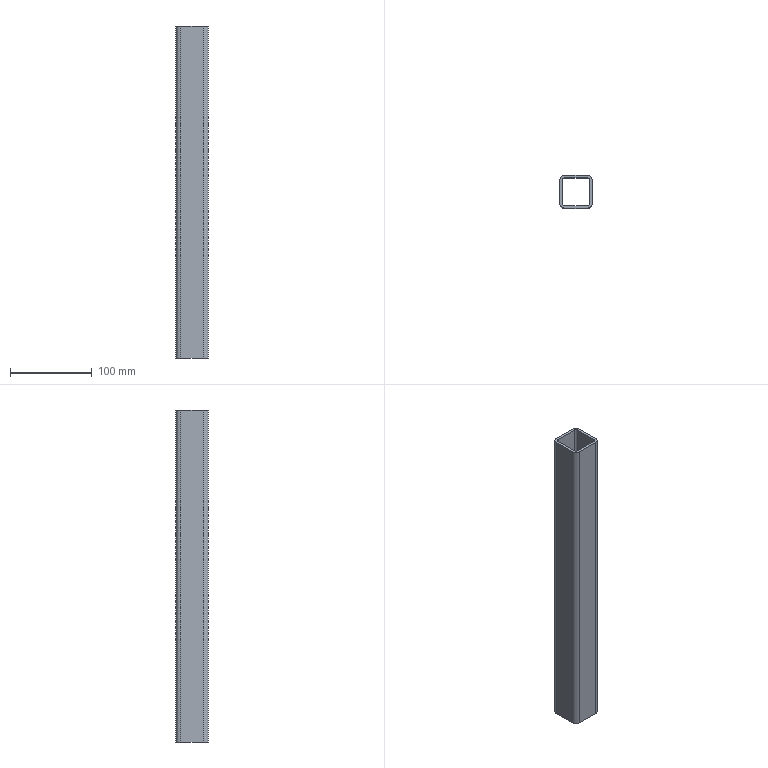Part | STEP file | SN10_003_008-08_TUBO_QUADRADO | 1 solid | 18 faces | box 40 x 40 x 407 mm | volume 171275 mm3 | plane 10 | cylinder 8 | commonest cylinder face diameters 6 x4 12 x4
STEP:
#1=CARTESIAN_POINT('',(0.,0.,0.));
#2=DIRECTION('',(0.,0.,1.));
#3=DIRECTION('',(1.,0.,0.));
#4=AXIS2_PLACEMENT_3D('',#1,#2,#3);
#5=CARTESIAN_POINT('',(2332.,-174.,20.));
#6=VERTEX_POINT('',#5);
#7=CARTESIAN_POINT('',(2326.,-180.,20.));
#8=VERTEX_POINT('',#7);
#9=CARTESIAN_POINT('',(2326.,-174.,20.));
#10=DIRECTION('',(0.,0.,-1.));
#11=DIRECTION('',(1.,0.,0.));
#12=AXIS2_PLACEMENT_3D('',#9,#10,#11);
#13=CIRCLE('',#12,6.);
#14=CARTESIAN_POINT('',(0.,0.,20.));
#15=DIRECTION('',(0.,0.,-1.));
#16=DIRECTION('',(-1.,0.,0.));
#17=AXIS2_PLACEMENT_3D('',#14,#15,#16);
#18=PLANE('',#17);
#19=CARTESIAN_POINT('',(-2326.,-174.));
#20=DIRECTION('',(-1.,0.));
#21=AXIS2_PLACEMENT_2D('',#19,#20);
#22=CIRCLE('',#21,6.);
#23=(GEOMETRIC_REPRESENTATION_CONTEXT(2)PARAMETRIC_REPRESENTATION_CONTEXT()REPRESENTATION_CONTEXT('',''));
#24=DEFINITIONAL_REPRESENTATION('',(#22),#23);
#25=PCURVE('',#18,#24);
#26=CARTESIAN_POINT('',(2326.,-174.,224.11));
#27=DIRECTION('',(0.,0.,-1.));
#28=DIRECTION('',(1.,0.,0.));
#29=AXIS2_PLACEMENT_3D('',#26,#27,#28);
#30=CYLINDRICAL_SURFACE('',#29,6.);
#31=CARTESIAN_POINT('',(0.,204.11));
#32=DIRECTION('',(1.,0.));
#33=VECTOR('',#32,1.);
#34=LINE('',#31,#33);
#35=(GEOMETRIC_REPRESENTATION_CONTEXT(2)PARAMETRIC_REPRESENTATION_CONTEXT()REPRESENTATION_CONTEXT('',''));
#36=DEFINITIONAL_REPRESENTATION('',(#34),#35);
#37=PCURVE('',#30,#36);
#38=SURFACE_CURVE('',#13,(#25,#37),.PCURVE_S1.);
#39=EDGE_CURVE('',#6,#8,#38,.T.);
#40=ORIENTED_EDGE('',*,*,#39,.T.);
#41=CARTESIAN_POINT('',(2298.,-180.,20.));
#42=VERTEX_POINT('',#41);
#43=CARTESIAN_POINT('',(2298.,-180.,20.));
#44=DIRECTION('',(1.,0.,0.));
#45=VECTOR('',#44,1.);
#46=LINE('',#43,#45);
#47=CARTESIAN_POINT('',(-2298.,-180.));
#48=DIRECTION('',(-1.,0.));
#49=VECTOR('',#48,1.);
#50=LINE('',#47,#49);
#51=(GEOMETRIC_REPRESENTATION_CONTEXT(2)PARAMETRIC_REPRESENTATION_CONTEXT()REPRESENTATION_CONTEXT('',''));
#52=DEFINITIONAL_REPRESENTATION('',(#50),#51);
#53=PCURVE('',#18,#52);
#54=CARTESIAN_POINT('',(2298.,-180.,20.));
#55=DIRECTION('',(0.,-1.,0.));
#56=DIRECTION('',(0.,0.,-1.));
#57=AXIS2_PLACEMENT_3D('',#54,#55,#56);
#58=PLANE('',#57);
#59=CARTESIAN_POINT('',(0.,0.));
#60=DIRECTION('',(0.,1.));
#61=VECTOR('',#60,1.);
#62=LINE('',#59,#61);
#63=(GEOMETRIC_REPRESENTATION_CONTEXT(2)PARAMETRIC_REPRESENTATION_CONTEXT()REPRESENTATION_CONTEXT('',''));
#64=DEFINITIONAL_REPRESENTATION('',(#62),#63);
#65=PCURVE('',#58,#64);
#66=SURFACE_CURVE('',#46,(#53,#65),.PCURVE_S1.);
#67=EDGE_CURVE('',#42,#8,#66,.T.);
#68=ORIENTED_EDGE('',*,*,#67,.F.);
#69=CARTESIAN_POINT('',(2292.,-174.,20.));
#70=VERTEX_POINT('',#69);
#71=CARTESIAN_POINT('',(2298.,-174.,20.));
#72=DIRECTION('',(0.,0.,-1.));
#73=DIRECTION('',(1.,0.,0.));
#74=AXIS2_PLACEMENT_3D('',#71,#72,#73);
#75=CIRCLE('',#74,6.);
#76=CARTESIAN_POINT('',(-2298.,-174.));
#77=DIRECTION('',(-1.,0.));
#78=AXIS2_PLACEMENT_2D('',#76,#77);
#79=CIRCLE('',#78,6.);
#80=(GEOMETRIC_REPRESENTATION_CONTEXT(2)PARAMETRIC_REPRESENTATION_CONTEXT()REPRESENTATION_CONTEXT('',''));
#81=DEFINITIONAL_REPRESENTATION('',(#79),#80);
#82=PCURVE('',#18,#81);
#83=CARTESIAN_POINT('',(2298.,-174.,224.11));
#84=DIRECTION('',(0.,0.,-1.));
#85=DIRECTION('',(0.,-1.,0.));
#86=AXIS2_PLACEMENT_3D('',#83,#84,#85);
#87=CYLINDRICAL_SURFACE('',#86,6.);
#88=CARTESIAN_POINT('',(-1.571,204.11));
#89=DIRECTION('',(1.,0.));
#90=VECTOR('',#89,1.);
#91=LINE('',#88,#90);
#92=(GEOMETRIC_REPRESENTATION_CONTEXT(2)PARAMETRIC_REPRESENTATION_CONTEXT()REPRESENTATION_CONTEXT('',''));
#93=DEFINITIONAL_REPRESENTATION('',(#91),#92);
#94=PCURVE('',#87,#93);
#95=SURFACE_CURVE('',#75,(#82,#94),.PCURVE_S1.);
#96=EDGE_CURVE('',#42,#70,#95,.T.);
#97=ORIENTED_EDGE('',*,*,#96,.T.);
#98=CARTESIAN_POINT('',(2292.,-146.,20.));
#99=VERTEX_POINT('',#98);
#100=CARTESIAN_POINT('',(2292.,-146.,20.));
#101=DIRECTION('',(0.,-1.,0.));
#102=VECTOR('',#101,1.);
#103=LINE('',#100,#102);
#104=CARTESIAN_POINT('',(-2292.,-146.));
#105=DIRECTION('',(0.,-1.));
#106=VECTOR('',#105,1.);
#107=LINE('',#104,#106);
#108=(GEOMETRIC_REPRESENTATION_CONTEXT(2)PARAMETRIC_REPRESENTATION_CONTEXT()REPRESENTATION_CONTEXT('',''));
#109=DEFINITIONAL_REPRESENTATION('',(#107),#108);
#110=PCURVE('',#18,#109);
#111=CARTESIAN_POINT('',(2292.,-146.,20.));
#112=DIRECTION('',(-1.,0.,0.));
#113=DIRECTION('',(0.,0.,1.));
#114=AXIS2_PLACEMENT_3D('',#111,#112,#113);
#115=PLANE('',#114);
#116=CARTESIAN_POINT('',(0.,0.));
#117=DIRECTION('',(0.,-1.));
#118=VECTOR('',#117,1.);
#119=LINE('',#116,#118);
#120=(GEOMETRIC_REPRESENTATION_CONTEXT(2)PARAMETRIC_REPRESENTATION_CONTEXT()REPRESENTATION_CONTEXT('',''));
#121=DEFINITIONAL_REPRESENTATION('',(#119),#120);
#122=PCURVE('',#115,#121);
#123=SURFACE_CURVE('',#103,(#110,#122),.PCURVE_S1.);
#124=EDGE_CURVE('',#99,#70,#123,.T.);
#125=ORIENTED_EDGE('',*,*,#124,.F.);
#126=CARTESIAN_POINT('',(2298.,-140.,20.));
#127=VERTEX_POINT('',#126);
#128=CARTESIAN_POINT('',(2298.,-146.,20.));
#129=DIRECTION('',(0.,0.,-1.));
#130=DIRECTION('',(1.,0.,0.));
#131=AXIS2_PLACEMENT_3D('',#128,#129,#130);
#132=CIRCLE('',#131,6.);
#133=CARTESIAN_POINT('',(-2298.,-146.));
#134=DIRECTION('',(-1.,0.));
#135=AXIS2_PLACEMENT_2D('',#133,#134);
#136=CIRCLE('',#135,6.);
#137=(GEOMETRIC_REPRESENTATION_CONTEXT(2)PARAMETRIC_REPRESENTATION_CONTEXT()REPRESENTATION_CONTEXT('',''));
#138=DEFINITIONAL_REPRESENTATION('',(#136),#137);
#139=PCURVE('',#18,#138);
#140=CARTESIAN_POINT('',(2298.,-146.,224.11));
#141=DIRECTION('',(0.,0.,-1.));
#142=DIRECTION('',(-1.,0.,0.));
#143=AXIS2_PLACEMENT_3D('',#140,#141,#142);
#144=CYLINDRICAL_SURFACE('',#143,6.);
#145=CARTESIAN_POINT('',(-3.142,204.11));
#146=DIRECTION('',(1.,0.));
#147=VECTOR('',#146,1.);
#148=LINE('',#145,#147);
#149=(GEOMETRIC_REPRESENTATION_CONTEXT(2)PARAMETRIC_REPRESENTATION_CONTEXT()REPRESENTATION_CONTEXT('',''));
#150=DEFINITIONAL_REPRESENTATION('',(#148),#149);
#151=PCURVE('',#144,#150);
#152=SURFACE_CURVE('',#132,(#139,#151),.PCURVE_S1.);
#153=EDGE_CURVE('',#99,#127,#152,.T.);
#154=ORIENTED_EDGE('',*,*,#153,.T.);
#155=CARTESIAN_POINT('',(2326.,-140.,20.));
#156=VERTEX_POINT('',#155);
#157=CARTESIAN_POINT('',(2326.,-140.,20.));
#158=DIRECTION('',(-1.,0.,0.));
#159=VECTOR('',#158,1.);
#160=LINE('',#157,#159);
#161=CARTESIAN_POINT('',(-2326.,-140.));
#162=DIRECTION('',(1.,0.));
#163=VECTOR('',#162,1.);
#164=LINE('',#161,#163);
#165=(GEOMETRIC_REPRESENTATION_CONTEXT(2)PARAMETRIC_REPRESENTATION_CONTEXT()REPRESENTATION_CONTEXT('',''));
#166=DEFINITIONAL_REPRESENTATION('',(#164),#165);
#167=PCURVE('',#18,#166);
#168=CARTESIAN_POINT('',(2326.,-140.,20.));
#169=DIRECTION('',(0.,1.,0.));
#170=DIRECTION('',(0.,0.,1.));
#171=AXIS2_PLACEMENT_3D('',#168,#169,#170);
#172=PLANE('',#171);
#173=CARTESIAN_POINT('',(0.,0.));
#174=DIRECTION('',(0.,-1.));
#175=VECTOR('',#174,1.);
#176=LINE('',#173,#175);
#177=(GEOMETRIC_REPRESENTATION_CONTEXT(2)PARAMETRIC_REPRESENTATION_CONTEXT()REPRESENTATION_CONTEXT('',''));
#178=DEFINITIONAL_REPRESENTATION('',(#176),#177);
#179=PCURVE('',#172,#178);
#180=SURFACE_CURVE('',#160,(#167,#179),.PCURVE_S1.);
#181=EDGE_CURVE('',#156,#127,#180,.T.);
#182=ORIENTED_EDGE('',*,*,#181,.F.);
#183=CARTESIAN_POINT('',(2332.,-146.,20.));
#184=VERTEX_POINT('',#183);
#185=CARTESIAN_POINT('',(2326.,-146.,20.));
#186=DIRECTION('',(0.,0.,-1.));
#187=DIRECTION('',(1.,0.,0.));
#188=AXIS2_PLACEMENT_3D('',#185,#186,#187);
#189=CIRCLE('',#188,6.);
#190=CARTESIAN_POINT('',(-2326.,-146.));
#191=DIRECTION('',(-1.,0.));
#192=AXIS2_PLACEMENT_2D('',#190,#191);
#193=CIRCLE('',#192,6.);
#194=(GEOMETRIC_REPRESENTATION_CONTEXT(2)PARAMETRIC_REPRESENTATION_CONTEXT()REPRESENTATION_CONTEXT('',''));
#195=DEFINITIONAL_REPRESENTATION('',(#193),#194);
#196=PCURVE('',#18,#195);
#197=CARTESIAN_POINT('',(2326.,-146.,224.11));
#198=DIRECTION('',(0.,0.,-1.));
#199=DIRECTION('',(0.,1.,0.));
#200=AXIS2_PLACEMENT_3D('',#197,#198,#199);
#201=CYLINDRICAL_SURFACE('',#200,6.);
#202=CARTESIAN_POINT('',(-4.712,204.11));
#203=DIRECTION('',(1.,0.));
#204=VECTOR('',#203,1.);
#205=LINE('',#202,#204);
#206=(GEOMETRIC_REPRESENTATION_CONTEXT(2)PARAMETRIC_REPRESENTATION_CONTEXT()REPRESENTATION_CONTEXT('',''));
#207=DEFINITIONAL_REPRESENTATION('',(#205),#206);
#208=PCURVE('',#201,#207);
#209=SURFACE_CURVE('',#189,(#196,#208),.PCURVE_S1.);
#210=EDGE_CURVE('',#156,#184,#209,.T.);
#211=ORIENTED_EDGE('',*,*,#210,.T.);
#212=CARTESIAN_POINT('',(2332.,-174.,20.));
#213=DIRECTION('',(0.,1.,0.));
#214=VECTOR('',#213,1.);
#215=LINE('',#212,#214);
#216=CARTESIAN_POINT('',(-2332.,-174.));
#217=DIRECTION('',(0.,1.));
#218=VECTOR('',#217,1.);
#219=LINE('',#216,#218);
#220=(GEOMETRIC_REPRESENTATION_CONTEXT(2)PARAMETRIC_REPRESENTATION_CONTEXT()REPRESENTATION_CONTEXT('',''));
#221=DEFINITIONAL_REPRESENTATION('',(#219),#220);
#222=PCURVE('',#18,#221);
#223=CARTESIAN_POINT('',(2332.,-174.,20.));
#224=DIRECTION('',(1.,0.,0.));
#225=DIRECTION('',(0.,0.,-1.));
#226=AXIS2_PLACEMENT_3D('',#223,#224,#225);
#227=PLANE('',#226);
#228=CARTESIAN_POINT('',(0.,0.));
#229=DIRECTION('',(0.,1.));
#230=VECTOR('',#229,1.);
#231=LINE('',#228,#230);
#232=(GEOMETRIC_REPRESENTATION_CONTEXT(2)PARAMETRIC_REPRESENTATION_CONTEXT()REPRESENTATION_CONTEXT('',''));
#233=DEFINITIONAL_REPRESENTATION('',(#231),#232);
#234=PCURVE('',#227,#233);
#235=SURFACE_CURVE('',#215,(#222,#234),.PCURVE_S1.);
#236=EDGE_CURVE('',#6,#184,#235,.T.);
#237=ORIENTED_EDGE('',*,*,#236,.F.);
#238=EDGE_LOOP('',(#40,#68,#97,#125,#154,#182,#211,#237));
#239=FACE_BOUND('',#238,.T.);
#240=CARTESIAN_POINT('',(2329.,-174.,20.));
#241=VERTEX_POINT('',#240);
#242=CARTESIAN_POINT('',(2329.,-146.,20.));
#243=VERTEX_POINT('',#242);
#244=CARTESIAN_POINT('',(2329.,-174.,20.));
#245=DIRECTION('',(0.,1.,0.));
#246=VECTOR('',#245,1.);
#247=LINE('',#244,#246);
#248=CARTESIAN_POINT('',(-2329.,-174.));
#249=DIRECTION('',(0.,1.));
#250=VECTOR('',#249,1.);
#251=LINE('',#248,#250);
#252=(GEOMETRIC_REPRESENTATION_CONTEXT(2)PARAMETRIC_REPRESENTATION_CONTEXT()REPRESENTATION_CONTEXT('',''));
#253=DEFINITIONAL_REPRESENTATION('',(#251),#252);
#254=PCURVE('',#18,#253);
#255=CARTESIAN_POINT('',(2329.,-174.,20.));
#256=DIRECTION('',(1.,0.,0.));
#257=DIRECTION('',(0.,0.,-1.));
#258=AXIS2_PLACEMENT_3D('',#255,#256,#257);
#259=PLANE('',#258);
#260=CARTESIAN_POINT('',(0.,0.));
#261=DIRECTION('',(0.,1.));
#262=VECTOR('',#261,1.);
#263=LINE('',#260,#262);
#264=(GEOMETRIC_REPRESENTATION_CONTEXT(2)PARAMETRIC_REPRESENTATION_CONTEXT()REPRESENTATION_CONTEXT('',''));
#265=DEFINITIONAL_REPRESENTATION('',(#263),#264);
#266=PCURVE('',#259,#265);
#267=SURFACE_CURVE('',#247,(#254,#266),.PCURVE_S1.);
#268=EDGE_CURVE('',#241,#243,#267,.T.);
#269=ORIENTED_EDGE('',*,*,#268,.T.);
#270=CARTESIAN_POINT('',(2326.,-143.,20.));
#271=VERTEX_POINT('',#270);
#272=CARTESIAN_POINT('',(2326.,-146.,20.));
#273=DIRECTION('',(0.,0.,-1.));
#274=DIRECTION('',(1.,0.,0.));
#275=AXIS2_PLACEMENT_3D('',#272,#273,#274);
#276=CIRCLE('',#275,3.);
#277=CARTESIAN_POINT('',(-2326.,-146.));
#278=DIRECTION('',(-1.,0.));
#279=AXIS2_PLACEMENT_2D('',#277,#278);
#280=CIRCLE('',#279,3.);
#281=(GEOMETRIC_REPRESENTATION_CONTEXT(2)PARAMETRIC_REPRESENTATION_CONTEXT()REPRESENTATION_CONTEXT('',''));
#282=DEFINITIONAL_REPRESENTATION('',(#280),#281);
#283=PCURVE('',#18,#282);
#284=CARTESIAN_POINT('',(2326.,-146.,224.11));
#285=DIRECTION('',(0.,0.,-1.));
#286=DIRECTION('',(0.,1.,0.));
#287=AXIS2_PLACEMENT_3D('',#284,#285,#286);
#288=CYLINDRICAL_SURFACE('',#287,3.);
#289=CARTESIAN_POINT('',(-4.712,204.11));
#290=DIRECTION('',(1.,0.));
#291=VECTOR('',#290,1.);
#292=LINE('',#289,#291);
#293=(GEOMETRIC_REPRESENTATION_CONTEXT(2)PARAMETRIC_REPRESENTATION_CONTEXT()REPRESENTATION_CONTEXT('',''));
#294=DEFINITIONAL_REPRESENTATION('',(#292),#293);
#295=PCURVE('',#288,#294);
#296=SURFACE_CURVE('',#276,(#283,#295),.PCURVE_S1.);
#297=EDGE_CURVE('',#271,#243,#296,.T.);
#298=ORIENTED_EDGE('',*,*,#297,.F.);
#299=CARTESIAN_POINT('',(2298.,-143.,20.));
#300=VERTEX_POINT('',#299);
#301=CARTESIAN_POINT('',(2326.,-143.,20.));
#302=DIRECTION('',(-1.,0.,0.));
#303=VECTOR('',#302,1.);
#304=LINE('',#301,#303);
#305=CARTESIAN_POINT('',(-2326.,-143.));
#306=DIRECTION('',(1.,0.));
#307=VECTOR('',#306,1.);
#308=LINE('',#305,#307);
#309=(GEOMETRIC_REPRESENTATION_CONTEXT(2)PARAMETRIC_REPRESENTATION_CONTEXT()REPRESENTATION_CONTEXT('',''));
#310=DEFINITIONAL_REPRESENTATION('',(#308),#309);
#311=PCURVE('',#18,#310);
#312=CARTESIAN_POINT('',(2326.,-143.,20.));
#313=DIRECTION('',(0.,1.,0.));
#314=DIRECTION('',(0.,0.,1.));
#315=AXIS2_PLACEMENT_3D('',#312,#313,#314);
#316=PLANE('',#315);
#317=CARTESIAN_POINT('',(0.,0.));
#318=DIRECTION('',(0.,-1.));
#319=VECTOR('',#318,1.);
#320=LINE('',#317,#319);
#321=(GEOMETRIC_REPRESENTATION_CONTEXT(2)PARAMETRIC_REPRESENTATION_CONTEXT()REPRESENTATION_CONTEXT('',''));
#322=DEFINITIONAL_REPRESENTATION('',(#320),#321);
#323=PCURVE('',#316,#322);
#324=SURFACE_CURVE('',#304,(#311,#323),.PCURVE_S1.);
#325=EDGE_CURVE('',#271,#300,#324,.T.);
#326=ORIENTED_EDGE('',*,*,#325,.T.);
#327=CARTESIAN_POINT('',(2295.,-146.,20.));
#328=VERTEX_POINT('',#327);
#329=CARTESIAN_POINT('',(2298.,-146.,20.));
#330=DIRECTION('',(0.,0.,-1.));
#331=DIRECTION('',(1.,0.,0.));
#332=AXIS2_PLACEMENT_3D('',#329,#330,#331);
#333=CIRCLE('',#332,3.);
#334=CARTESIAN_POINT('',(-2298.,-146.));
#335=DIRECTION('',(-1.,0.));
#336=AXIS2_PLACEMENT_2D('',#334,#335);
#337=CIRCLE('',#336,3.);
#338=(GEOMETRIC_REPRESENTATION_CONTEXT(2)PARAMETRIC_REPRESENTATION_CONTEXT()REPRESENTATION_CONTEXT('',''));
#339=DEFINITIONAL_REPRESENTATION('',(#337),#338);
#340=PCURVE('',#18,#339);
#341=CARTESIAN_POINT('',(2298.,-146.,224.11));
#342=DIRECTION('',(0.,0.,-1.));
#343=DIRECTION('',(-1.,0.,0.));
#344=AXIS2_PLACEMENT_3D('',#341,#342,#343);
#345=CYLINDRICAL_SURFACE('',#344,3.);
#346=CARTESIAN_POINT('',(-3.142,204.11));
#347=DIRECTION('',(1.,0.));
#348=VECTOR('',#347,1.);
#349=LINE('',#346,#348);
#350=(GEOMETRIC_REPRESENTATION_CONTEXT(2)PARAMETRIC_REPRESENTATION_CONTEXT()REPRESENTATION_CONTEXT('',''));
#351=DEFINITIONAL_REPRESENTATION('',(#349),#350);
#352=PCURVE('',#345,#351);
#353=SURFACE_CURVE('',#333,(#340,#352),.PCURVE_S1.);
#354=EDGE_CURVE('',#328,#300,#353,.T.);
#355=ORIENTED_EDGE('',*,*,#354,.F.);
#356=CARTESIAN_POINT('',(2295.,-174.,20.));
#357=VERTEX_POINT('',#356);
#358=CARTESIAN_POINT('',(2295.,-146.,20.));
#359=DIRECTION('',(0.,-1.,0.));
#360=VECTOR('',#359,1.);
#361=LINE('',#358,#360);
#362=CARTESIAN_POINT('',(-2295.,-146.));
#363=DIRECTION('',(0.,-1.));
#364=VECTOR('',#363,1.);
#365=LINE('',#362,#364);
#366=(GEOMETRIC_REPRESENTATION_CONTEXT(2)PARAMETRIC_REPRESENTATION_CONTEXT()REPRESENTATION_CONTEXT('',''));
#367=DEFINITIONAL_REPRESENTATION('',(#365),#366);
#368=PCURVE('',#18,#367);
#369=CARTESIAN_POINT('',(2295.,-146.,20.));
#370=DIRECTION('',(-1.,0.,0.));
#371=DIRECTION('',(0.,0.,1.));
#372=AXIS2_PLACEMENT_3D('',#369,#370,#371);
#373=PLANE('',#372);
#374=CARTESIAN_POINT('',(0.,0.));
#375=DIRECTION('',(0.,-1.));
#376=VECTOR('',#375,1.);
#377=LINE('',#374,#376);
#378=(GEOMETRIC_REPRESENTATION_CONTEXT(2)PARAMETRIC_REPRESENTATION_CONTEXT()REPRESENTATION_CONTEXT('',''));
#379=DEFINITIONAL_REPRESENTATION('',(#377),#378);
#380=PCURVE('',#373,#379);
#381=SURFACE_CURVE('',#361,(#368,#380),.PCURVE_S1.);
#382=EDGE_CURVE('',#328,#357,#381,.T.);
#383=ORIENTED_EDGE('',*,*,#382,.T.);
#384=CARTESIAN_POINT('',(2298.,-177.,20.));
#385=VERTEX_POINT('',#384);
#386=CARTESIAN_POINT('',(2298.,-174.,20.));
#387=DIRECTION('',(0.,0.,-1.));
#388=DIRECTION('',(1.,0.,0.));
#389=AXIS2_PLACEMENT_3D('',#386,#387,#388);
#390=CIRCLE('',#389,3.);
#391=CARTESIAN_POINT('',(-2298.,-174.));
#392=DIRECTION('',(-1.,0.));
#393=AXIS2_PLACEMENT_2D('',#391,#392);
#394=CIRCLE('',#393,3.);
#395=(GEOMETRIC_REPRESENTATION_CONTEXT(2)PARAMETRIC_REPRESENTATION_CONTEXT()REPRESENTATION_CONTEXT('',''));
#396=DEFINITIONAL_REPRESENTATION('',(#394),#395);
#397=PCURVE('',#18,#396);
#398=CARTESIAN_POINT('',(2298.,-174.,224.11));
#399=DIRECTION('',(0.,0.,-1.));
#400=DIRECTION('',(0.,-1.,0.));
#401=AXIS2_PLACEMENT_3D('',#398,#399,#400);
#402=CYLINDRICAL_SURFACE('',#401,3.);
#403=CARTESIAN_POINT('',(-1.571,204.11));
#404=DIRECTION('',(1.,0.));
#405=VECTOR('',#404,1.);
#406=LINE('',#403,#405);
#407=(GEOMETRIC_REPRESENTATION_CONTEXT(2)PARAMETRIC_REPRESENTATION_CONTEXT()REPRESENTATION_CONTEXT('',''));
#408=DEFINITIONAL_REPRESENTATION('',(#406),#407);
#409=PCURVE('',#402,#408);
#410=SURFACE_CURVE('',#390,(#397,#409),.PCURVE_S1.);
#411=EDGE_CURVE('',#385,#357,#410,.T.);
#412=ORIENTED_EDGE('',*,*,#411,.F.);
#413=CARTESIAN_POINT('',(2326.,-177.,20.));
#414=VERTEX_POINT('',#413);
#415=CARTESIAN_POINT('',(2298.,-177.,20.));
#416=DIRECTION('',(1.,0.,0.));
#417=VECTOR('',#416,1.);
#418=LINE('',#415,#417);
#419=CARTESIAN_POINT('',(-2298.,-177.));
#420=DIRECTION('',(-1.,0.));
#421=VECTOR('',#420,1.);
#422=LINE('',#419,#421);
#423=(GEOMETRIC_REPRESENTATION_CONTEXT(2)PARAMETRIC_REPRESENTATION_CONTEXT()REPRESENTATION_CONTEXT('',''));
#424=DEFINITIONAL_REPRESENTATION('',(#422),#423);
#425=PCURVE('',#18,#424);
#426=CARTESIAN_POINT('',(2298.,-177.,20.));
#427=DIRECTION('',(0.,-1.,0.));
#428=DIRECTION('',(0.,0.,-1.));
#429=AXIS2_PLACEMENT_3D('',#426,#427,#428);
#430=PLANE('',#429);
#431=CARTESIAN_POINT('',(0.,0.));
#432=DIRECTION('',(0.,1.));
#433=VECTOR('',#432,1.);
#434=LINE('',#431,#433);
#435=(GEOMETRIC_REPRESENTATION_CONTEXT(2)PARAMETRIC_REPRESENTATION_CONTEXT()REPRESENTATION_CONTEXT('',''));
#436=DEFINITIONAL_REPRESENTATION('',(#434),#435);
#437=PCURVE('',#430,#436);
#438=SURFACE_CURVE('',#418,(#425,#437),.PCURVE_S1.);
#439=EDGE_CURVE('',#385,#414,#438,.T.);
#440=ORIENTED_EDGE('',*,*,#439,.T.);
#441=CARTESIAN_POINT('',(2326.,-174.,20.));
#442=DIRECTION('',(0.,0.,-1.));
#443=DIRECTION('',(1.,0.,0.));
#444=AXIS2_PLACEMENT_3D('',#441,#442,#443);
#445=CIRCLE('',#444,3.);
#446=CARTESIAN_POINT('',(-2326.,-174.));
#447=DIRECTION('',(-1.,0.));
#448=AXIS2_PLACEMENT_2D('',#446,#447);
#449=CIRCLE('',#448,3.);
#450=(GEOMETRIC_REPRESENTATION_CONTEXT(2)PARAMETRIC_REPRESENTATION_CONTEXT()REPRESENTATION_CONTEXT('',''));
#451=DEFINITIONAL_REPRESENTATION('',(#449),#450);
#452=PCURVE('',#18,#451);
#453=CARTESIAN_POINT('',(2326.,-174.,224.11));
#454=DIRECTION('',(0.,0.,-1.));
#455=DIRECTION('',(1.,0.,0.));
#456=AXIS2_PLACEMENT_3D('',#453,#454,#455);
#457=CYLINDRICAL_SURFACE('',#456,3.);
#458=CARTESIAN_POINT('',(0.,204.11));
#459=DIRECTION('',(1.,0.));
#460=VECTOR('',#459,1.);
#461=LINE('',#458,#460);
#462=(GEOMETRIC_REPRESENTATION_CONTEXT(2)PARAMETRIC_REPRESENTATION_CONTEXT()REPRESENTATION_CONTEXT('',''));
#463=DEFINITIONAL_REPRESENTATION('',(#461),#462);
#464=PCURVE('',#457,#463);
#465=SURFACE_CURVE('',#445,(#452,#464),.PCURVE_S1.);
#466=EDGE_CURVE('',#241,#414,#465,.T.);
#467=ORIENTED_EDGE('',*,*,#466,.F.);
#468=EDGE_LOOP('',(#269,#298,#326,#355,#383,#412,#440,#467));
#469=FACE_BOUND('',#468,.T.);
#470=ADVANCED_FACE('',(#239,#469),#18,.T.);
#471=CARTESIAN_POINT('',(2326.,-180.,427.));
#472=VERTEX_POINT('',#471);
#473=CARTESIAN_POINT('',(2326.,-180.,427.));
#474=DIRECTION('',(0.,0.,-1.));
#475=VECTOR('',#474,1.);
#476=LINE('',#473,#475);
#477=CARTESIAN_POINT('',(1.571,-202.89));
#478=DIRECTION('',(0.,1.));
#479=VECTOR('',#478,1.);
#480=LINE('',#477,#479);
#481=(GEOMETRIC_REPRESENTATION_CONTEXT(2)PARAMETRIC_REPRESENTATION_CONTEXT()REPRESENTATION_CONTEXT('',''));
#482=DEFINITIONAL_REPRESENTATION('',(#480),#481);
#483=PCURVE('',#30,#482);
#484=CARTESIAN_POINT('',(-407.,28.));
#485=DIRECTION('',(1.,0.));
#486=VECTOR('',#485,1.);
#487=LINE('',#484,#486);
#488=(GEOMETRIC_REPRESENTATION_CONTEXT(2)PARAMETRIC_REPRESENTATION_CONTEXT()REPRESENTATION_CONTEXT('',''));
#489=DEFINITIONAL_REPRESENTATION('',(#487),#488);
#490=PCURVE('',#58,#489);
#491=SURFACE_CURVE('',#476,(#483,#490),.PCURVE_S1.);
#492=EDGE_CURVE('',#472,#8,#491,.T.);
#493=ORIENTED_EDGE('',*,*,#492,.T.);
#494=ORIENTED_EDGE('',*,*,#39,.F.);
#495=CARTESIAN_POINT('',(2332.,-174.,427.));
#496=VERTEX_POINT('',#495);
#497=CARTESIAN_POINT('',(2332.,-174.,427.));
#498=DIRECTION('',(0.,0.,-1.));
#499=VECTOR('',#498,1.);
#500=LINE('',#497,#499);
#501=CARTESIAN_POINT('',(0.,-202.89));
#502=DIRECTION('',(0.,1.));
#503=VECTOR('',#502,1.);
#504=LINE('',#501,#503);
#505=(GEOMETRIC_REPRESENTATION_CONTEXT(2)PARAMETRIC_REPRESENTATION_CONTEXT()REPRESENTATION_CONTEXT('',''));
#506=DEFINITIONAL_REPRESENTATION('',(#504),#505);
#507=PCURVE('',#30,#506);
#508=CARTESIAN_POINT('',(-407.,0.));
#509=DIRECTION('',(1.,0.));
#510=VECTOR('',#509,1.);
#511=LINE('',#508,#510);
#512=(GEOMETRIC_REPRESENTATION_CONTEXT(2)PARAMETRIC_REPRESENTATION_CONTEXT()REPRESENTATION_CONTEXT('',''));
#513=DEFINITIONAL_REPRESENTATION('',(#511),#512);
#514=PCURVE('',#227,#513);
#515=SURFACE_CURVE('',#500,(#507,#514),.PCURVE_S1.);
#516=EDGE_CURVE('',#496,#6,#515,.T.);
#517=ORIENTED_EDGE('',*,*,#516,.F.);
#518=CARTESIAN_POINT('',(2326.,-174.,427.));
#519=DIRECTION('',(0.,0.,-1.));
#520=DIRECTION('',(1.,0.,0.));
#521=AXIS2_PLACEMENT_3D('',#518,#519,#520);
#522=CIRCLE('',#521,6.);
#523=CARTESIAN_POINT('',(0.,-202.89));
#524=DIRECTION('',(1.,0.));
#525=VECTOR('',#524,1.);
#526=LINE('',#523,#525);
#527=(GEOMETRIC_REPRESENTATION_CONTEXT(2)PARAMETRIC_REPRESENTATION_CONTEXT()REPRESENTATION_CONTEXT('',''));
#528=DEFINITIONAL_REPRESENTATION('',(#526),#527);
#529=PCURVE('',#30,#528);
#530=CARTESIAN_POINT('',(-20.,-146.,427.));
#531=DIRECTION('',(0.,0.,1.));
#532=DIRECTION('',(1.,0.,0.));
#533=AXIS2_PLACEMENT_3D('',#530,#531,#532);
#534=PLANE('',#533);
#535=CARTESIAN_POINT('',(2352.,-28.));
#536=CARTESIAN_POINT('',(2352.,-38.392));
#537=CARTESIAN_POINT('',(2343.,-33.196));
#538=CARTESIAN_POINT('',(2334.,-28.));
#539=CARTESIAN_POINT('',(2343.,-22.804));
#540=CARTESIAN_POINT('',(2352.,-17.608));
#541=CARTESIAN_POINT('',(2352.,-28.));
#542=(BOUNDED_CURVE()B_SPLINE_CURVE(2,(#535,#536,#537,#538,#539,#540,#541),.UNSPECIFIED.,.T.,.F.)B_SPLINE_CURVE_WITH_KNOTS((1,2,2,2,2,1),(-2.094,0.,2.094,4.189,6.283,8.378),.UNSPECIFIED.)CURVE()GEOMETRIC_REPRESENTATION_ITEM()RATIONAL_B_SPLINE_CURVE((1.,0.5,1.,0.5,1.,0.5,1.))REPRESENTATION_ITEM(''));
#543=(GEOMETRIC_REPRESENTATION_CONTEXT(2)PARAMETRIC_REPRESENTATION_CONTEXT()REPRESENTATION_CONTEXT('',''));
#544=DEFINITIONAL_REPRESENTATION('',(#542),#543);
#545=PCURVE('',#534,#544);
#546=SURFACE_CURVE('',#522,(#529,#545),.PCURVE_S1.);
#547=EDGE_CURVE('',#496,#472,#546,.T.);
#548=ORIENTED_EDGE('',*,*,#547,.T.);
#549=EDGE_LOOP('',(#493,#494,#517,#548));
#550=FACE_BOUND('',#549,.T.);
#551=ADVANCED_FACE('',(#550),#30,.T.);
#552=CARTESIAN_POINT('',(2298.,-180.,427.));
#553=VERTEX_POINT('',#552);
#554=CARTESIAN_POINT('',(2298.,-180.,20.));
#555=DIRECTION('',(0.,0.,1.));
#556=VECTOR('',#555,1.);
#557=LINE('',#554,#556);
#558=CARTESIAN_POINT('',(0.,0.));
#559=DIRECTION('',(-1.,0.));
#560=VECTOR('',#559,1.);
#561=LINE('',#558,#560);
#562=(GEOMETRIC_REPRESENTATION_CONTEXT(2)PARAMETRIC_REPRESENTATION_CONTEXT()REPRESENTATION_CONTEXT('',''));
#563=DEFINITIONAL_REPRESENTATION('',(#561),#562);
#564=PCURVE('',#58,#563);
#565=CARTESIAN_POINT('',(0.,204.11));
#566=DIRECTION('',(0.,-1.));
#567=VECTOR('',#566,1.);
#568=LINE('',#565,#567);
#569=(GEOMETRIC_REPRESENTATION_CONTEXT(2)PARAMETRIC_REPRESENTATION_CONTEXT()REPRESENTATION_CONTEXT('',''));
#570=DEFINITIONAL_REPRESENTATION('',(#568),#569);
#571=PCURVE('',#87,#570);
#572=SURFACE_CURVE('',#557,(#564,#571),.PCURVE_S1.);
#573=EDGE_CURVE('',#42,#553,#572,.T.);
#574=ORIENTED_EDGE('',*,*,#573,.F.);
#575=ORIENTED_EDGE('',*,*,#67,.T.);
#576=ORIENTED_EDGE('',*,*,#492,.F.);
#577=CARTESIAN_POINT('',(2298.,-180.,427.));
#578=DIRECTION('',(1.,0.,0.));
#579=VECTOR('',#578,1.);
#580=LINE('',#577,#579);
#581=CARTESIAN_POINT('',(-407.,0.));
#582=DIRECTION('',(0.,1.));
#583=VECTOR('',#582,1.);
#584=LINE('',#581,#583);
#585=(GEOMETRIC_REPRESENTATION_CONTEXT(2)PARAMETRIC_REPRESENTATION_CONTEXT()REPRESENTATION_CONTEXT('',''));
#586=DEFINITIONAL_REPRESENTATION('',(#584),#585);
#587=PCURVE('',#58,#586);
#588=CARTESIAN_POINT('',(2318.,-34.));
#589=DIRECTION('',(1.,0.));
#590=VECTOR('',#589,1.);
#591=LINE('',#588,#590);
#592=(GEOMETRIC_REPRESENTATION_CONTEXT(2)PARAMETRIC_REPRESENTATION_CONTEXT()REPRESENTATION_CONTEXT('',''));
#593=DEFINITIONAL_REPRESENTATION('',(#591),#592);
#594=PCURVE('',#534,#593);
#595=SURFACE_CURVE('',#580,(#587,#594),.PCURVE_S1.);
#596=EDGE_CURVE('',#553,#472,#595,.T.);
#597=ORIENTED_EDGE('',*,*,#596,.F.);
#598=EDGE_LOOP('',(#574,#575,#576,#597));
#599=FACE_BOUND('',#598,.T.);
#600=ADVANCED_FACE('',(#599),#58,.T.);
#601=CARTESIAN_POINT('',(2292.,-174.,427.));
#602=VERTEX_POINT('',#601);
#603=CARTESIAN_POINT('',(2292.,-174.,427.));
#604=DIRECTION('',(0.,0.,-1.));
#605=VECTOR('',#604,1.);
#606=LINE('',#603,#605);
#607=CARTESIAN_POINT('',(1.571,-202.89));
#608=DIRECTION('',(0.,1.));
#609=VECTOR('',#608,1.);
#610=LINE('',#607,#609);
#611=(GEOMETRIC_REPRESENTATION_CONTEXT(2)PARAMETRIC_REPRESENTATION_CONTEXT()REPRESENTATION_CONTEXT('',''));
#612=DEFINITIONAL_REPRESENTATION('',(#610),#611);
#613=PCURVE('',#87,#612);
#614=CARTESIAN_POINT('',(407.,-28.));
#615=DIRECTION('',(-1.,0.));
#616=VECTOR('',#615,1.);
#617=LINE('',#614,#616);
#618=(GEOMETRIC_REPRESENTATION_CONTEXT(2)PARAMETRIC_REPRESENTATION_CONTEXT()REPRESENTATION_CONTEXT('',''));
#619=DEFINITIONAL_REPRESENTATION('',(#617),#618);
#620=PCURVE('',#115,#619);
#621=SURFACE_CURVE('',#606,(#613,#620),.PCURVE_S1.);
#622=EDGE_CURVE('',#602,#70,#621,.T.);
#623=ORIENTED_EDGE('',*,*,#622,.T.);
#624=ORIENTED_EDGE('',*,*,#96,.F.);
#625=ORIENTED_EDGE('',*,*,#573,.T.);
#626=CARTESIAN_POINT('',(2298.,-174.,427.));
#627=DIRECTION('',(0.,0.,-1.));
#628=DIRECTION('',(1.,0.,0.));
#629=AXIS2_PLACEMENT_3D('',#626,#627,#628);
#630=CIRCLE('',#629,6.);
#631=CARTESIAN_POINT('',(-1.571,-202.89));
#632=DIRECTION('',(1.,0.));
#633=VECTOR('',#632,1.);
#634=LINE('',#631,#633);
#635=(GEOMETRIC_REPRESENTATION_CONTEXT(2)PARAMETRIC_REPRESENTATION_CONTEXT()REPRESENTATION_CONTEXT('',''));
#636=DEFINITIONAL_REPRESENTATION('',(#634),#635);
#637=PCURVE('',#87,#636);
#638=CARTESIAN_POINT('',(2324.,-28.));
#639=CARTESIAN_POINT('',(2324.,-38.392));
#640=CARTESIAN_POINT('',(2315.,-33.196));
#641=CARTESIAN_POINT('',(2306.,-28.));
#642=CARTESIAN_POINT('',(2315.,-22.804));
#643=CARTESIAN_POINT('',(2324.,-17.608));
#644=CARTESIAN_POINT('',(2324.,-28.));
#645=(BOUNDED_CURVE()B_SPLINE_CURVE(2,(#638,#639,#640,#641,#642,#643,#644),.UNSPECIFIED.,.T.,.F.)B_SPLINE_CURVE_WITH_KNOTS((1,2,2,2,2,1),(-2.094,0.,2.094,4.189,6.283,8.378),.UNSPECIFIED.)CURVE()GEOMETRIC_REPRESENTATION_ITEM()RATIONAL_B_SPLINE_CURVE((1.,0.5,1.,0.5,1.,0.5,1.))REPRESENTATION_ITEM(''));
#646=(GEOMETRIC_REPRESENTATION_CONTEXT(2)PARAMETRIC_REPRESENTATION_CONTEXT()REPRESENTATION_CONTEXT('',''));
#647=DEFINITIONAL_REPRESENTATION('',(#645),#646);
#648=PCURVE('',#534,#647);
#649=SURFACE_CURVE('',#630,(#637,#648),.PCURVE_S1.);
#650=EDGE_CURVE('',#553,#602,#649,.T.);
#651=ORIENTED_EDGE('',*,*,#650,.T.);
#652=EDGE_LOOP('',(#623,#624,#625,#651));
#653=FACE_BOUND('',#652,.T.);
#654=ADVANCED_FACE('',(#653),#87,.T.);
#655=CARTESIAN_POINT('',(2292.,-146.,427.));
#656=VERTEX_POINT('',#655);
#657=CARTESIAN_POINT('',(2292.,-146.,20.));
#658=DIRECTION('',(0.,0.,1.));
#659=VECTOR('',#658,1.);
#660=LINE('',#657,#659);
#661=CARTESIAN_POINT('',(0.,0.));
#662=DIRECTION('',(1.,0.));
#663=VECTOR('',#662,1.);
#664=LINE('',#661,#663);
#665=(GEOMETRIC_REPRESENTATION_CONTEXT(2)PARAMETRIC_REPRESENTATION_CONTEXT()REPRESENTATION_CONTEXT('',''));
#666=DEFINITIONAL_REPRESENTATION('',(#664),#665);
#667=PCURVE('',#115,#666);
#668=CARTESIAN_POINT('',(0.,204.11));
#669=DIRECTION('',(0.,-1.));
#670=VECTOR('',#669,1.);
#671=LINE('',#668,#670);
#672=(GEOMETRIC_REPRESENTATION_CONTEXT(2)PARAMETRIC_REPRESENTATION_CONTEXT()REPRESENTATION_CONTEXT('',''));
#673=DEFINITIONAL_REPRESENTATION('',(#671),#672);
#674=PCURVE('',#144,#673);
#675=SURFACE_CURVE('',#660,(#667,#674),.PCURVE_S1.);
#676=EDGE_CURVE('',#99,#656,#675,.T.);
#677=ORIENTED_EDGE('',*,*,#676,.F.);
#678=ORIENTED_EDGE('',*,*,#124,.T.);
#679=ORIENTED_EDGE('',*,*,#622,.F.);
#680=CARTESIAN_POINT('',(2292.,-146.,427.));
#681=DIRECTION('',(0.,-1.,0.));
#682=VECTOR('',#681,1.);
#683=LINE('',#680,#682);
#684=CARTESIAN_POINT('',(407.,0.));
#685=DIRECTION('',(0.,-1.));
#686=VECTOR('',#685,1.);
#687=LINE('',#684,#686);
#688=(GEOMETRIC_REPRESENTATION_CONTEXT(2)PARAMETRIC_REPRESENTATION_CONTEXT()REPRESENTATION_CONTEXT('',''));
#689=DEFINITIONAL_REPRESENTATION('',(#687),#688);
#690=PCURVE('',#115,#689);
#691=CARTESIAN_POINT('',(2312.,0.));
#692=DIRECTION('',(0.,-1.));
#693=VECTOR('',#692,1.);
#694=LINE('',#691,#693);
#695=(GEOMETRIC_REPRESENTATION_CONTEXT(2)PARAMETRIC_REPRESENTATION_CONTEXT()REPRESENTATION_CONTEXT('',''));
#696=DEFINITIONAL_REPRESENTATION('',(#694),#695);
#697=PCURVE('',#534,#696);
#698=SURFACE_CURVE('',#683,(#690,#697),.PCURVE_S1.);
#699=EDGE_CURVE('',#656,#602,#698,.T.);
#700=ORIENTED_EDGE('',*,*,#699,.F.);
#701=EDGE_LOOP('',(#677,#678,#679,#700));
#702=FACE_BOUND('',#701,.T.);
#703=ADVANCED_FACE('',(#702),#115,.T.);
#704=CARTESIAN_POINT('',(2298.,-140.,427.));
#705=VERTEX_POINT('',#704);
#706=CARTESIAN_POINT('',(2298.,-140.,427.));
#707=DIRECTION('',(0.,0.,-1.));
#708=VECTOR('',#707,1.);
#709=LINE('',#706,#708);
#710=CARTESIAN_POINT('',(1.571,-202.89));
#711=DIRECTION('',(0.,1.));
#712=VECTOR('',#711,1.);
#713=LINE('',#710,#712);
#714=(GEOMETRIC_REPRESENTATION_CONTEXT(2)PARAMETRIC_REPRESENTATION_CONTEXT()REPRESENTATION_CONTEXT('',''));
#715=DEFINITIONAL_REPRESENTATION('',(#713),#714);
#716=PCURVE('',#144,#715);
#717=CARTESIAN_POINT('',(407.,-28.));
#718=DIRECTION('',(-1.,0.));
#719=VECTOR('',#718,1.);
#720=LINE('',#717,#719);
#721=(GEOMETRIC_REPRESENTATION_CONTEXT(2)PARAMETRIC_REPRESENTATION_CONTEXT()REPRESENTATION_CONTEXT('',''));
#722=DEFINITIONAL_REPRESENTATION('',(#720),#721);
#723=PCURVE('',#172,#722);
#724=SURFACE_CURVE('',#709,(#716,#723),.PCURVE_S1.);
#725=EDGE_CURVE('',#705,#127,#724,.T.);
#726=ORIENTED_EDGE('',*,*,#725,.T.);
#727=ORIENTED_EDGE('',*,*,#153,.F.);
#728=ORIENTED_EDGE('',*,*,#676,.T.);
#729=CARTESIAN_POINT('',(2298.,-146.,427.));
#730=DIRECTION('',(0.,0.,-1.));
#731=DIRECTION('',(1.,0.,0.));
#732=AXIS2_PLACEMENT_3D('',#729,#730,#731);
#733=CIRCLE('',#732,6.);
#734=CARTESIAN_POINT('',(-3.142,-202.89));
#735=DIRECTION('',(1.,0.));
#736=VECTOR('',#735,1.);
#737=LINE('',#734,#736);
#738=(GEOMETRIC_REPRESENTATION_CONTEXT(2)PARAMETRIC_REPRESENTATION_CONTEXT()REPRESENTATION_CONTEXT('',''));
#739=DEFINITIONAL_REPRESENTATION('',(#737),#738);
#740=PCURVE('',#144,#739);
#741=CARTESIAN_POINT('',(2324.,0.));
#742=CARTESIAN_POINT('',(2324.,-10.392));
#743=CARTESIAN_POINT('',(2315.,-5.196));
#744=CARTESIAN_POINT('',(2306.,0.));
#745=CARTESIAN_POINT('',(2315.,5.196));
#746=CARTESIAN_POINT('',(2324.,10.392));
#747=CARTESIAN_POINT('',(2324.,0.));
#748=(BOUNDED_CURVE()B_SPLINE_CURVE(2,(#741,#742,#743,#744,#745,#746,#747),.UNSPECIFIED.,.T.,.F.)B_SPLINE_CURVE_WITH_KNOTS((1,2,2,2,2,1),(-2.094,0.,2.094,4.189,6.283,8.378),.UNSPECIFIED.)CURVE()GEOMETRIC_REPRESENTATION_ITEM()RATIONAL_B_SPLINE_CURVE((1.,0.5,1.,0.5,1.,0.5,1.))REPRESENTATION_ITEM(''));
#749=(GEOMETRIC_REPRESENTATION_CONTEXT(2)PARAMETRIC_REPRESENTATION_CONTEXT()REPRESENTATION_CONTEXT('',''));
#750=DEFINITIONAL_REPRESENTATION('',(#748),#749);
#751=PCURVE('',#534,#750);
#752=SURFACE_CURVE('',#733,(#740,#751),.PCURVE_S1.);
#753=EDGE_CURVE('',#656,#705,#752,.T.);
#754=ORIENTED_EDGE('',*,*,#753,.T.);
#755=EDGE_LOOP('',(#726,#727,#728,#754));
#756=FACE_BOUND('',#755,.T.);
#757=ADVANCED_FACE('',(#756),#144,.T.);
#758=CARTESIAN_POINT('',(2326.,-140.,427.));
#759=VERTEX_POINT('',#758);
#760=CARTESIAN_POINT('',(2326.,-140.,20.));
#761=DIRECTION('',(0.,0.,1.));
#762=VECTOR('',#761,1.);
#763=LINE('',#760,#762);
#764=CARTESIAN_POINT('',(0.,0.));
#765=DIRECTION('',(1.,0.));
#766=VECTOR('',#765,1.);
#767=LINE('',#764,#766);
#768=(GEOMETRIC_REPRESENTATION_CONTEXT(2)PARAMETRIC_REPRESENTATION_CONTEXT()REPRESENTATION_CONTEXT('',''));
#769=DEFINITIONAL_REPRESENTATION('',(#767),#768);
#770=PCURVE('',#172,#769);
#771=CARTESIAN_POINT('',(0.,204.11));
#772=DIRECTION('',(0.,-1.));
#773=VECTOR('',#772,1.);
#774=LINE('',#771,#773);
#775=(GEOMETRIC_REPRESENTATION_CONTEXT(2)PARAMETRIC_REPRESENTATION_CONTEXT()REPRESENTATION_CONTEXT('',''));
#776=DEFINITIONAL_REPRESENTATION('',(#774),#775);
#777=PCURVE('',#201,#776);
#778=SURFACE_CURVE('',#763,(#770,#777),.PCURVE_S1.);
#779=EDGE_CURVE('',#156,#759,#778,.T.);
#780=ORIENTED_EDGE('',*,*,#779,.F.);
#781=ORIENTED_EDGE('',*,*,#181,.T.);
#782=ORIENTED_EDGE('',*,*,#725,.F.);
#783=CARTESIAN_POINT('',(2326.,-140.,427.));
#784=DIRECTION('',(-1.,0.,0.));
#785=VECTOR('',#784,1.);
#786=LINE('',#783,#785);
#787=CARTESIAN_POINT('',(407.,0.));
#788=DIRECTION('',(0.,-1.));
#789=VECTOR('',#788,1.);
#790=LINE('',#787,#789);
#791=(GEOMETRIC_REPRESENTATION_CONTEXT(2)PARAMETRIC_REPRESENTATION_CONTEXT()REPRESENTATION_CONTEXT('',''));
#792=DEFINITIONAL_REPRESENTATION('',(#790),#791);
#793=PCURVE('',#172,#792);
#794=CARTESIAN_POINT('',(2346.,6.));
#795=DIRECTION('',(-1.,0.));
#796=VECTOR('',#795,1.);
#797=LINE('',#794,#796);
#798=(GEOMETRIC_REPRESENTATION_CONTEXT(2)PARAMETRIC_REPRESENTATION_CONTEXT()REPRESENTATION_CONTEXT('',''));
#799=DEFINITIONAL_REPRESENTATION('',(#797),#798);
#800=PCURVE('',#534,#799);
#801=SURFACE_CURVE('',#786,(#793,#800),.PCURVE_S1.);
#802=EDGE_CURVE('',#759,#705,#801,.T.);
#803=ORIENTED_EDGE('',*,*,#802,.F.);
#804=EDGE_LOOP('',(#780,#781,#782,#803));
#805=FACE_BOUND('',#804,.T.);
#806=ADVANCED_FACE('',(#805),#172,.T.);
#807=CARTESIAN_POINT('',(2332.,-146.,427.));
#808=VERTEX_POINT('',#807);
#809=CARTESIAN_POINT('',(2332.,-146.,427.));
#810=DIRECTION('',(0.,0.,-1.));
#811=VECTOR('',#810,1.);
#812=LINE('',#809,#811);
#813=CARTESIAN_POINT('',(1.571,-202.89));
#814=DIRECTION('',(0.,1.));
#815=VECTOR('',#814,1.);
#816=LINE('',#813,#815);
#817=(GEOMETRIC_REPRESENTATION_CONTEXT(2)PARAMETRIC_REPRESENTATION_CONTEXT()REPRESENTATION_CONTEXT('',''));
#818=DEFINITIONAL_REPRESENTATION('',(#816),#817);
#819=PCURVE('',#201,#818);
#820=CARTESIAN_POINT('',(-407.,28.));
#821=DIRECTION('',(1.,0.));
#822=VECTOR('',#821,1.);
#823=LINE('',#820,#822);
#824=(GEOMETRIC_REPRESENTATION_CONTEXT(2)PARAMETRIC_REPRESENTATION_CONTEXT()REPRESENTATION_CONTEXT('',''));
#825=DEFINITIONAL_REPRESENTATION('',(#823),#824);
#826=PCURVE('',#227,#825);
#827=SURFACE_CURVE('',#812,(#819,#826),.PCURVE_S1.);
#828=EDGE_CURVE('',#808,#184,#827,.T.);
#829=ORIENTED_EDGE('',*,*,#828,.T.);
#830=ORIENTED_EDGE('',*,*,#210,.F.);
#831=ORIENTED_EDGE('',*,*,#779,.T.);
#832=CARTESIAN_POINT('',(2326.,-146.,427.));
#833=DIRECTION('',(0.,0.,-1.));
#834=DIRECTION('',(1.,0.,0.));
#835=AXIS2_PLACEMENT_3D('',#832,#833,#834);
#836=CIRCLE('',#835,6.);
#837=CARTESIAN_POINT('',(-4.712,-202.89));
#838=DIRECTION('',(1.,0.));
#839=VECTOR('',#838,1.);
#840=LINE('',#837,#839);
#841=(GEOMETRIC_REPRESENTATION_CONTEXT(2)PARAMETRIC_REPRESENTATION_CONTEXT()REPRESENTATION_CONTEXT('',''));
#842=DEFINITIONAL_REPRESENTATION('',(#840),#841);
#843=PCURVE('',#201,#842);
#844=CARTESIAN_POINT('',(2352.,0.));
#845=CARTESIAN_POINT('',(2352.,-10.392));
#846=CARTESIAN_POINT('',(2343.,-5.196));
#847=CARTESIAN_POINT('',(2334.,0.));
#848=CARTESIAN_POINT('',(2343.,5.196));
#849=CARTESIAN_POINT('',(2352.,10.392));
#850=CARTESIAN_POINT('',(2352.,0.));
#851=(BOUNDED_CURVE()B_SPLINE_CURVE(2,(#844,#845,#846,#847,#848,#849,#850),.UNSPECIFIED.,.T.,.F.)B_SPLINE_CURVE_WITH_KNOTS((1,2,2,2,2,1),(-2.094,0.,2.094,4.189,6.283,8.378),.UNSPECIFIED.)CURVE()GEOMETRIC_REPRESENTATION_ITEM()RATIONAL_B_SPLINE_CURVE((1.,0.5,1.,0.5,1.,0.5,1.))REPRESENTATION_ITEM(''));
#852=(GEOMETRIC_REPRESENTATION_CONTEXT(2)PARAMETRIC_REPRESENTATION_CONTEXT()REPRESENTATION_CONTEXT('',''));
#853=DEFINITIONAL_REPRESENTATION('',(#851),#852);
#854=PCURVE('',#534,#853);
#855=SURFACE_CURVE('',#836,(#843,#854),.PCURVE_S1.);
#856=EDGE_CURVE('',#759,#808,#855,.T.);
#857=ORIENTED_EDGE('',*,*,#856,.T.);
#858=EDGE_LOOP('',(#829,#830,#831,#857));
#859=FACE_BOUND('',#858,.T.);
#860=ADVANCED_FACE('',(#859),#201,.T.);
#861=ORIENTED_EDGE('',*,*,#516,.T.);
#862=ORIENTED_EDGE('',*,*,#236,.T.);
#863=ORIENTED_EDGE('',*,*,#828,.F.);
#864=CARTESIAN_POINT('',(2332.,-174.,427.));
#865=DIRECTION('',(0.,1.,0.));
#866=VECTOR('',#865,1.);
#867=LINE('',#864,#866);
#868=CARTESIAN_POINT('',(-407.,0.));
#869=DIRECTION('',(0.,1.));
#870=VECTOR('',#869,1.);
#871=LINE('',#868,#870);
#872=(GEOMETRIC_REPRESENTATION_CONTEXT(2)PARAMETRIC_REPRESENTATION_CONTEXT()REPRESENTATION_CONTEXT('',''));
#873=DEFINITIONAL_REPRESENTATION('',(#871),#872);
#874=PCURVE('',#227,#873);
#875=CARTESIAN_POINT('',(2352.,-28.));
#876=DIRECTION('',(0.,1.));
#877=VECTOR('',#876,1.);
#878=LINE('',#875,#877);
#879=(GEOMETRIC_REPRESENTATION_CONTEXT(2)PARAMETRIC_REPRESENTATION_CONTEXT()REPRESENTATION_CONTEXT('',''));
#880=DEFINITIONAL_REPRESENTATION('',(#878),#879);
#881=PCURVE('',#534,#880);
#882=SURFACE_CURVE('',#867,(#874,#881),.PCURVE_S1.);
#883=EDGE_CURVE('',#496,#808,#882,.T.);
#884=ORIENTED_EDGE('',*,*,#883,.F.);
#885=EDGE_LOOP('',(#861,#862,#863,#884));
#886=FACE_BOUND('',#885,.T.);
#887=ADVANCED_FACE('',(#886),#227,.T.);
#888=ORIENTED_EDGE('',*,*,#856,.F.);
#889=ORIENTED_EDGE('',*,*,#802,.T.);
#890=ORIENTED_EDGE('',*,*,#753,.F.);
#891=ORIENTED_EDGE('',*,*,#699,.T.);
#892=ORIENTED_EDGE('',*,*,#650,.F.);
#893=ORIENTED_EDGE('',*,*,#596,.T.);
#894=ORIENTED_EDGE('',*,*,#547,.F.);
#895=ORIENTED_EDGE('',*,*,#883,.T.);
#896=EDGE_LOOP('',(#888,#889,#890,#891,#892,#893,#894,#895));
#897=FACE_BOUND('',#896,.T.);
#898=CARTESIAN_POINT('',(2298.,-177.,427.));
#899=VERTEX_POINT('',#898);
#900=CARTESIAN_POINT('',(2326.,-177.,427.));
#901=VERTEX_POINT('',#900);
#902=CARTESIAN_POINT('',(2298.,-177.,427.));
#903=DIRECTION('',(1.,0.,0.));
#904=VECTOR('',#903,1.);
#905=LINE('',#902,#904);
#906=CARTESIAN_POINT('',(2318.,-31.));
#907=DIRECTION('',(1.,0.));
#908=VECTOR('',#907,1.);
#909=LINE('',#906,#908);
#910=(GEOMETRIC_REPRESENTATION_CONTEXT(2)PARAMETRIC_REPRESENTATION_CONTEXT()REPRESENTATION_CONTEXT('',''));
#911=DEFINITIONAL_REPRESENTATION('',(#909),#910);
#912=PCURVE('',#534,#911);
#913=CARTESIAN_POINT('',(-407.,0.));
#914=DIRECTION('',(0.,1.));
#915=VECTOR('',#914,1.);
#916=LINE('',#913,#915);
#917=(GEOMETRIC_REPRESENTATION_CONTEXT(2)PARAMETRIC_REPRESENTATION_CONTEXT()REPRESENTATION_CONTEXT('',''));
#918=DEFINITIONAL_REPRESENTATION('',(#916),#917);
#919=PCURVE('',#430,#918);
#920=SURFACE_CURVE('',#905,(#912,#919),.PCURVE_S1.);
#921=EDGE_CURVE('',#899,#901,#920,.T.);
#922=ORIENTED_EDGE('',*,*,#921,.F.);
#923=CARTESIAN_POINT('',(2295.,-174.,427.));
#924=VERTEX_POINT('',#923);
#925=CARTESIAN_POINT('',(2298.,-174.,427.));
#926=DIRECTION('',(0.,0.,1.));
#927=DIRECTION('',(1.,0.,0.));
#928=AXIS2_PLACEMENT_3D('',#925,#926,#927);
#929=CIRCLE('',#928,3.);
#930=CARTESIAN_POINT('',(2318.,-28.));
#931=DIRECTION('',(1.,0.));
#932=AXIS2_PLACEMENT_2D('',#930,#931);
#933=CIRCLE('',#932,3.);
#934=(GEOMETRIC_REPRESENTATION_CONTEXT(2)PARAMETRIC_REPRESENTATION_CONTEXT()REPRESENTATION_CONTEXT('',''));
#935=DEFINITIONAL_REPRESENTATION('',(#933),#934);
#936=PCURVE('',#534,#935);
#937=CARTESIAN_POINT('',(4.712,-202.89));
#938=DIRECTION('',(-1.,0.));
#939=VECTOR('',#938,1.);
#940=LINE('',#937,#939);
#941=(GEOMETRIC_REPRESENTATION_CONTEXT(2)PARAMETRIC_REPRESENTATION_CONTEXT()REPRESENTATION_CONTEXT('',''));
#942=DEFINITIONAL_REPRESENTATION('',(#940),#941);
#943=PCURVE('',#402,#942);
#944=SURFACE_CURVE('',#929,(#936,#943),.PCURVE_S1.);
#945=EDGE_CURVE('',#924,#899,#944,.T.);
#946=ORIENTED_EDGE('',*,*,#945,.F.);
#947=CARTESIAN_POINT('',(2295.,-146.,427.));
#948=VERTEX_POINT('',#947);
#949=CARTESIAN_POINT('',(2295.,-146.,427.));
#950=DIRECTION('',(0.,-1.,0.));
#951=VECTOR('',#950,1.);
#952=LINE('',#949,#951);
#953=CARTESIAN_POINT('',(2315.,0.));
#954=DIRECTION('',(0.,-1.));
#955=VECTOR('',#954,1.);
#956=LINE('',#953,#955);
#957=(GEOMETRIC_REPRESENTATION_CONTEXT(2)PARAMETRIC_REPRESENTATION_CONTEXT()REPRESENTATION_CONTEXT('',''));
#958=DEFINITIONAL_REPRESENTATION('',(#956),#957);
#959=PCURVE('',#534,#958);
#960=CARTESIAN_POINT('',(407.,0.));
#961=DIRECTION('',(0.,-1.));
#962=VECTOR('',#961,1.);
#963=LINE('',#960,#962);
#964=(GEOMETRIC_REPRESENTATION_CONTEXT(2)PARAMETRIC_REPRESENTATION_CONTEXT()REPRESENTATION_CONTEXT('',''));
#965=DEFINITIONAL_REPRESENTATION('',(#963),#964);
#966=PCURVE('',#373,#965);
#967=SURFACE_CURVE('',#952,(#959,#966),.PCURVE_S1.);
#968=EDGE_CURVE('',#948,#924,#967,.T.);
#969=ORIENTED_EDGE('',*,*,#968,.F.);
#970=CARTESIAN_POINT('',(2298.,-143.,427.));
#971=VERTEX_POINT('',#970);
#972=CARTESIAN_POINT('',(2298.,-146.,427.));
#973=DIRECTION('',(0.,0.,1.));
#974=DIRECTION('',(1.,0.,0.));
#975=AXIS2_PLACEMENT_3D('',#972,#973,#974);
#976=CIRCLE('',#975,3.);
#977=CARTESIAN_POINT('',(2318.,0.));
#978=DIRECTION('',(1.,0.));
#979=AXIS2_PLACEMENT_2D('',#977,#978);
#980=CIRCLE('',#979,3.);
#981=(GEOMETRIC_REPRESENTATION_CONTEXT(2)PARAMETRIC_REPRESENTATION_CONTEXT()REPRESENTATION_CONTEXT('',''));
#982=DEFINITIONAL_REPRESENTATION('',(#980),#981);
#983=PCURVE('',#534,#982);
#984=CARTESIAN_POINT('',(3.142,-202.89));
#985=DIRECTION('',(-1.,0.));
#986=VECTOR('',#985,1.);
#987=LINE('',#984,#986);
#988=(GEOMETRIC_REPRESENTATION_CONTEXT(2)PARAMETRIC_REPRESENTATION_CONTEXT()REPRESENTATION_CONTEXT('',''));
#989=DEFINITIONAL_REPRESENTATION('',(#987),#988);
#990=PCURVE('',#345,#989);
#991=SURFACE_CURVE('',#976,(#983,#990),.PCURVE_S1.);
#992=EDGE_CURVE('',#971,#948,#991,.T.);
#993=ORIENTED_EDGE('',*,*,#992,.F.);
#994=CARTESIAN_POINT('',(2326.,-143.,427.));
#995=VERTEX_POINT('',#994);
#996=CARTESIAN_POINT('',(2326.,-143.,427.));
#997=DIRECTION('',(-1.,0.,0.));
#998=VECTOR('',#997,1.);
#999=LINE('',#996,#998);
#1000=CARTESIAN_POINT('',(2346.,3.));
#1001=DIRECTION('',(-1.,0.));
#1002=VECTOR('',#1001,1.);
#1003=LINE('',#1000,#1002);
#1004=(GEOMETRIC_REPRESENTATION_CONTEXT(2)PARAMETRIC_REPRESENTATION_CONTEXT()REPRESENTATION_CONTEXT('',''));
#1005=DEFINITIONAL_REPRESENTATION('',(#1003),#1004);
#1006=PCURVE('',#534,#1005);
#1007=CARTESIAN_POINT('',(407.,0.));
#1008=DIRECTION('',(0.,-1.));
#1009=VECTOR('',#1008,1.);
#1010=LINE('',#1007,#1009);
#1011=(GEOMETRIC_REPRESENTATION_CONTEXT(2)PARAMETRIC_REPRESENTATION_CONTEXT()REPRESENTATION_CONTEXT('',''));
#1012=DEFINITIONAL_REPRESENTATION('',(#1010),#1011);
#1013=PCURVE('',#316,#1012);
#1014=SURFACE_CURVE('',#999,(#1006,#1013),.PCURVE_S1.);
#1015=EDGE_CURVE('',#995,#971,#1014,.T.);
#1016=ORIENTED_EDGE('',*,*,#1015,.F.);
#1017=CARTESIAN_POINT('',(2329.,-146.,427.));
#1018=VERTEX_POINT('',#1017);
#1019=CARTESIAN_POINT('',(2326.,-146.,427.));
#1020=DIRECTION('',(0.,0.,1.));
#1021=DIRECTION('',(1.,0.,0.));
#1022=AXIS2_PLACEMENT_3D('',#1019,#1020,#1021);
#1023=CIRCLE('',#1022,3.);
#1024=CARTESIAN_POINT('',(2346.,0.));
#1025=DIRECTION('',(1.,0.));
#1026=AXIS2_PLACEMENT_2D('',#1024,#1025);
#1027=CIRCLE('',#1026,3.);
#1028=(GEOMETRIC_REPRESENTATION_CONTEXT(2)PARAMETRIC_REPRESENTATION_CONTEXT()REPRESENTATION_CONTEXT('',''));
#1029=DEFINITIONAL_REPRESENTATION('',(#1027),#1028);
#1030=PCURVE('',#534,#1029);
#1031=CARTESIAN_POINT('',(1.571,-202.89));
#1032=DIRECTION('',(-1.,0.));
#1033=VECTOR('',#1032,1.);
#1034=LINE('',#1031,#1033);
#1035=(GEOMETRIC_REPRESENTATION_CONTEXT(2)PARAMETRIC_REPRESENTATION_CONTEXT()REPRESENTATION_CONTEXT('',''));
#1036=DEFINITIONAL_REPRESENTATION('',(#1034),#1035);
#1037=PCURVE('',#288,#1036);
#1038=SURFACE_CURVE('',#1023,(#1030,#1037),.PCURVE_S1.);
#1039=EDGE_CURVE('',#1018,#995,#1038,.T.);
#1040=ORIENTED_EDGE('',*,*,#1039,.F.);
#1041=CARTESIAN_POINT('',(2329.,-174.,427.));
#1042=VERTEX_POINT('',#1041);
#1043=CARTESIAN_POINT('',(2329.,-174.,427.));
#1044=DIRECTION('',(0.,1.,0.));
#1045=VECTOR('',#1044,1.);
#1046=LINE('',#1043,#1045);
#1047=CARTESIAN_POINT('',(2349.,-28.));
#1048=DIRECTION('',(0.,1.));
#1049=VECTOR('',#1048,1.);
#1050=LINE('',#1047,#1049);
#1051=(GEOMETRIC_REPRESENTATION_CONTEXT(2)PARAMETRIC_REPRESENTATION_CONTEXT()REPRESENTATION_CONTEXT('',''));
#1052=DEFINITIONAL_REPRESENTATION('',(#1050),#1051);
#1053=PCURVE('',#534,#1052);
#1054=CARTESIAN_POINT('',(-407.,0.));
#1055=DIRECTION('',(0.,1.));
#1056=VECTOR('',#1055,1.);
#1057=LINE('',#1054,#1056);
#1058=(GEOMETRIC_REPRESENTATION_CONTEXT(2)PARAMETRIC_REPRESENTATION_CONTEXT()REPRESENTATION_CONTEXT('',''));
#1059=DEFINITIONAL_REPRESENTATION('',(#1057),#1058);
#1060=PCURVE('',#259,#1059);
#1061=SURFACE_CURVE('',#1046,(#1053,#1060),.PCURVE_S1.);
#1062=EDGE_CURVE('',#1042,#1018,#1061,.T.);
#1063=ORIENTED_EDGE('',*,*,#1062,.F.);
#1064=CARTESIAN_POINT('',(2326.,-174.,427.));
#1065=DIRECTION('',(0.,0.,1.));
#1066=DIRECTION('',(1.,0.,0.));
#1067=AXIS2_PLACEMENT_3D('',#1064,#1065,#1066);
#1068=CIRCLE('',#1067,3.);
#1069=CARTESIAN_POINT('',(2346.,-28.));
#1070=DIRECTION('',(1.,0.));
#1071=AXIS2_PLACEMENT_2D('',#1069,#1070);
#1072=CIRCLE('',#1071,3.);
#1073=(GEOMETRIC_REPRESENTATION_CONTEXT(2)PARAMETRIC_REPRESENTATION_CONTEXT()REPRESENTATION_CONTEXT('',''));
#1074=DEFINITIONAL_REPRESENTATION('',(#1072),#1073);
#1075=PCURVE('',#534,#1074);
#1076=CARTESIAN_POINT('',(6.283,-202.89));
#1077=DIRECTION('',(-1.,0.));
#1078=VECTOR('',#1077,1.);
#1079=LINE('',#1076,#1078);
#1080=(GEOMETRIC_REPRESENTATION_CONTEXT(2)PARAMETRIC_REPRESENTATION_CONTEXT()REPRESENTATION_CONTEXT('',''));
#1081=DEFINITIONAL_REPRESENTATION('',(#1079),#1080);
#1082=PCURVE('',#457,#1081);
#1083=SURFACE_CURVE('',#1068,(#1075,#1082),.PCURVE_S1.);
#1084=EDGE_CURVE('',#901,#1042,#1083,.T.);
#1085=ORIENTED_EDGE('',*,*,#1084,.F.);
#1086=EDGE_LOOP('',(#922,#946,#969,#993,#1016,#1040,#1063,#1085));
#1087=FACE_BOUND('',#1086,.T.);
#1088=ADVANCED_FACE('',(#897,#1087),#534,.T.);
#1089=CARTESIAN_POINT('',(2326.,-177.,427.));
#1090=DIRECTION('',(0.,0.,-1.));
#1091=VECTOR('',#1090,1.);
#1092=LINE('',#1089,#1091);
#1093=CARTESIAN_POINT('',(1.571,-202.89));
#1094=DIRECTION('',(0.,1.));
#1095=VECTOR('',#1094,1.);
#1096=LINE('',#1093,#1095);
#1097=(GEOMETRIC_REPRESENTATION_CONTEXT(2)PARAMETRIC_REPRESENTATION_CONTEXT()REPRESENTATION_CONTEXT('',''));
#1098=DEFINITIONAL_REPRESENTATION('',(#1096),#1097);
#1099=PCURVE('',#457,#1098);
#1100=CARTESIAN_POINT('',(-407.,28.));
#1101=DIRECTION('',(1.,0.));
#1102=VECTOR('',#1101,1.);
#1103=LINE('',#1100,#1102);
#1104=(GEOMETRIC_REPRESENTATION_CONTEXT(2)PARAMETRIC_REPRESENTATION_CONTEXT()REPRESENTATION_CONTEXT('',''));
#1105=DEFINITIONAL_REPRESENTATION('',(#1103),#1104);
#1106=PCURVE('',#430,#1105);
#1107=SURFACE_CURVE('',#1092,(#1099,#1106),.PCURVE_S1.);
#1108=EDGE_CURVE('',#901,#414,#1107,.T.);
#1109=ORIENTED_EDGE('',*,*,#1108,.T.);
#1110=ORIENTED_EDGE('',*,*,#466,.F.);
#1111=CARTESIAN_POINT('',(2329.,-174.,427.));
#1112=DIRECTION('',(0.,0.,-1.));
#1113=VECTOR('',#1112,1.);
#1114=LINE('',#1111,#1113);
#1115=CARTESIAN_POINT('',(0.,-202.89));
#1116=DIRECTION('',(0.,1.));
#1117=VECTOR('',#1116,1.);
#1118=LINE('',#1115,#1117);
#1119=(GEOMETRIC_REPRESENTATION_CONTEXT(2)PARAMETRIC_REPRESENTATION_CONTEXT()REPRESENTATION_CONTEXT('',''));
#1120=DEFINITIONAL_REPRESENTATION('',(#1118),#1119);
#1121=PCURVE('',#457,#1120);
#1122=CARTESIAN_POINT('',(-407.,0.));
#1123=DIRECTION('',(1.,0.));
#1124=VECTOR('',#1123,1.);
#1125=LINE('',#1122,#1124);
#1126=(GEOMETRIC_REPRESENTATION_CONTEXT(2)PARAMETRIC_REPRESENTATION_CONTEXT()REPRESENTATION_CONTEXT('',''));
#1127=DEFINITIONAL_REPRESENTATION('',(#1125),#1126);
#1128=PCURVE('',#259,#1127);
#1129=SURFACE_CURVE('',#1114,(#1121,#1128),.PCURVE_S1.);
#1130=EDGE_CURVE('',#1042,#241,#1129,.T.);
#1131=ORIENTED_EDGE('',*,*,#1130,.F.);
#1132=ORIENTED_EDGE('',*,*,#1084,.F.);
#1133=EDGE_LOOP('',(#1109,#1110,#1131,#1132));
#1134=FACE_BOUND('',#1133,.F.);
#1135=ADVANCED_FACE('',(#1134),#457,.F.);
#1136=ORIENTED_EDGE('',*,*,#921,.T.);
#1137=ORIENTED_EDGE('',*,*,#1108,.T.);
#1138=ORIENTED_EDGE('',*,*,#439,.F.);
#1139=CARTESIAN_POINT('',(2298.,-177.,20.));
#1140=DIRECTION('',(0.,0.,1.));
#1141=VECTOR('',#1140,1.);
#1142=LINE('',#1139,#1141);
#1143=CARTESIAN_POINT('',(0.,0.));
#1144=DIRECTION('',(-1.,0.));
#1145=VECTOR('',#1144,1.);
#1146=LINE('',#1143,#1145);
#1147=(GEOMETRIC_REPRESENTATION_CONTEXT(2)PARAMETRIC_REPRESENTATION_CONTEXT()REPRESENTATION_CONTEXT('',''));
#1148=DEFINITIONAL_REPRESENTATION('',(#1146),#1147);
#1149=PCURVE('',#430,#1148);
#1150=CARTESIAN_POINT('',(0.,204.11));
#1151=DIRECTION('',(0.,-1.));
#1152=VECTOR('',#1151,1.);
#1153=LINE('',#1150,#1152);
#1154=(GEOMETRIC_REPRESENTATION_CONTEXT(2)PARAMETRIC_REPRESENTATION_CONTEXT()REPRESENTATION_CONTEXT('',''));
#1155=DEFINITIONAL_REPRESENTATION('',(#1153),#1154);
#1156=PCURVE('',#402,#1155);
#1157=SURFACE_CURVE('',#1142,(#1149,#1156),.PCURVE_S1.);
#1158=EDGE_CURVE('',#385,#899,#1157,.T.);
#1159=ORIENTED_EDGE('',*,*,#1158,.T.);
#1160=EDGE_LOOP('',(#1136,#1137,#1138,#1159));
#1161=FACE_BOUND('',#1160,.T.);
#1162=ADVANCED_FACE('',(#1161),#430,.F.);
#1163=CARTESIAN_POINT('',(2295.,-174.,427.));
#1164=DIRECTION('',(0.,0.,-1.));
#1165=VECTOR('',#1164,1.);
#1166=LINE('',#1163,#1165);
#1167=CARTESIAN_POINT('',(1.571,-202.89));
#1168=DIRECTION('',(0.,1.));
#1169=VECTOR('',#1168,1.);
#1170=LINE('',#1167,#1169);
#1171=(GEOMETRIC_REPRESENTATION_CONTEXT(2)PARAMETRIC_REPRESENTATION_CONTEXT()REPRESENTATION_CONTEXT('',''));
#1172=DEFINITIONAL_REPRESENTATION('',(#1170),#1171);
#1173=PCURVE('',#402,#1172);
#1174=CARTESIAN_POINT('',(407.,-28.));
#1175=DIRECTION('',(-1.,0.));
#1176=VECTOR('',#1175,1.);
#1177=LINE('',#1174,#1176);
#1178=(GEOMETRIC_REPRESENTATION_CONTEXT(2)PARAMETRIC_REPRESENTATION_CONTEXT()REPRESENTATION_CONTEXT('',''));
#1179=DEFINITIONAL_REPRESENTATION('',(#1177),#1178);
#1180=PCURVE('',#373,#1179);
#1181=SURFACE_CURVE('',#1166,(#1173,#1180),.PCURVE_S1.);
#1182=EDGE_CURVE('',#924,#357,#1181,.T.);
#1183=ORIENTED_EDGE('',*,*,#1182,.T.);
#1184=ORIENTED_EDGE('',*,*,#411,.F.);
#1185=ORIENTED_EDGE('',*,*,#1158,.T.);
#1186=ORIENTED_EDGE('',*,*,#945,.F.);
#1187=EDGE_LOOP('',(#1183,#1184,#1185,#1186));
#1188=FACE_BOUND('',#1187,.F.);
#1189=ADVANCED_FACE('',(#1188),#402,.F.);
#1190=ORIENTED_EDGE('',*,*,#968,.T.);
#1191=ORIENTED_EDGE('',*,*,#1182,.T.);
#1192=ORIENTED_EDGE('',*,*,#382,.F.);
#1193=CARTESIAN_POINT('',(2295.,-146.,20.));
#1194=DIRECTION('',(0.,0.,1.));
#1195=VECTOR('',#1194,1.);
#1196=LINE('',#1193,#1195);
#1197=CARTESIAN_POINT('',(0.,0.));
#1198=DIRECTION('',(1.,0.));
#1199=VECTOR('',#1198,1.);
#1200=LINE('',#1197,#1199);
#1201=(GEOMETRIC_REPRESENTATION_CONTEXT(2)PARAMETRIC_REPRESENTATION_CONTEXT()REPRESENTATION_CONTEXT('',''));
#1202=DEFINITIONAL_REPRESENTATION('',(#1200),#1201);
#1203=PCURVE('',#373,#1202);
#1204=CARTESIAN_POINT('',(0.,204.11));
#1205=DIRECTION('',(0.,-1.));
#1206=VECTOR('',#1205,1.);
#1207=LINE('',#1204,#1206);
#1208=(GEOMETRIC_REPRESENTATION_CONTEXT(2)PARAMETRIC_REPRESENTATION_CONTEXT()REPRESENTATION_CONTEXT('',''));
#1209=DEFINITIONAL_REPRESENTATION('',(#1207),#1208);
#1210=PCURVE('',#345,#1209);
#1211=SURFACE_CURVE('',#1196,(#1203,#1210),.PCURVE_S1.);
#1212=EDGE_CURVE('',#328,#948,#1211,.T.);
#1213=ORIENTED_EDGE('',*,*,#1212,.T.);
#1214=EDGE_LOOP('',(#1190,#1191,#1192,#1213));
#1215=FACE_BOUND('',#1214,.T.);
#1216=ADVANCED_FACE('',(#1215),#373,.F.);
#1217=CARTESIAN_POINT('',(2298.,-143.,427.));
#1218=DIRECTION('',(0.,0.,-1.));
#1219=VECTOR('',#1218,1.);
#1220=LINE('',#1217,#1219);
#1221=CARTESIAN_POINT('',(1.571,-202.89));
#1222=DIRECTION('',(0.,1.));
#1223=VECTOR('',#1222,1.);
#1224=LINE('',#1221,#1223);
#1225=(GEOMETRIC_REPRESENTATION_CONTEXT(2)PARAMETRIC_REPRESENTATION_CONTEXT()REPRESENTATION_CONTEXT('',''));
#1226=DEFINITIONAL_REPRESENTATION('',(#1224),#1225);
#1227=PCURVE('',#345,#1226);
#1228=CARTESIAN_POINT('',(407.,-28.));
#1229=DIRECTION('',(-1.,0.));
#1230=VECTOR('',#1229,1.);
#1231=LINE('',#1228,#1230);
#1232=(GEOMETRIC_REPRESENTATION_CONTEXT(2)PARAMETRIC_REPRESENTATION_CONTEXT()REPRESENTATION_CONTEXT('',''));
#1233=DEFINITIONAL_REPRESENTATION('',(#1231),#1232);
#1234=PCURVE('',#316,#1233);
#1235=SURFACE_CURVE('',#1220,(#1227,#1234),.PCURVE_S1.);
#1236=EDGE_CURVE('',#971,#300,#1235,.T.);
#1237=ORIENTED_EDGE('',*,*,#1236,.T.);
#1238=ORIENTED_EDGE('',*,*,#354,.F.);
#1239=ORIENTED_EDGE('',*,*,#1212,.T.);
#1240=ORIENTED_EDGE('',*,*,#992,.F.);
#1241=EDGE_LOOP('',(#1237,#1238,#1239,#1240));
#1242=FACE_BOUND('',#1241,.F.);
#1243=ADVANCED_FACE('',(#1242),#345,.F.);
#1244=ORIENTED_EDGE('',*,*,#1015,.T.);
#1245=ORIENTED_EDGE('',*,*,#1236,.T.);
#1246=ORIENTED_EDGE('',*,*,#325,.F.);
#1247=CARTESIAN_POINT('',(2326.,-143.,20.));
#1248=DIRECTION('',(0.,0.,1.));
#1249=VECTOR('',#1248,1.);
#1250=LINE('',#1247,#1249);
#1251=CARTESIAN_POINT('',(0.,0.));
#1252=DIRECTION('',(1.,0.));
#1253=VECTOR('',#1252,1.);
#1254=LINE('',#1251,#1253);
#1255=(GEOMETRIC_REPRESENTATION_CONTEXT(2)PARAMETRIC_REPRESENTATION_CONTEXT()REPRESENTATION_CONTEXT('',''));
#1256=DEFINITIONAL_REPRESENTATION('',(#1254),#1255);
#1257=PCURVE('',#316,#1256);
#1258=CARTESIAN_POINT('',(0.,204.11));
#1259=DIRECTION('',(0.,-1.));
#1260=VECTOR('',#1259,1.);
#1261=LINE('',#1258,#1260);
#1262=(GEOMETRIC_REPRESENTATION_CONTEXT(2)PARAMETRIC_REPRESENTATION_CONTEXT()REPRESENTATION_CONTEXT('',''));
#1263=DEFINITIONAL_REPRESENTATION('',(#1261),#1262);
#1264=PCURVE('',#288,#1263);
#1265=SURFACE_CURVE('',#1250,(#1257,#1264),.PCURVE_S1.);
#1266=EDGE_CURVE('',#271,#995,#1265,.T.);
#1267=ORIENTED_EDGE('',*,*,#1266,.T.);
#1268=EDGE_LOOP('',(#1244,#1245,#1246,#1267));
#1269=FACE_BOUND('',#1268,.T.);
#1270=ADVANCED_FACE('',(#1269),#316,.F.);
#1271=CARTESIAN_POINT('',(2329.,-146.,427.));
#1272=DIRECTION('',(0.,0.,-1.));
#1273=VECTOR('',#1272,1.);
#1274=LINE('',#1271,#1273);
#1275=CARTESIAN_POINT('',(1.571,-202.89));
#1276=DIRECTION('',(0.,1.));
#1277=VECTOR('',#1276,1.);
#1278=LINE('',#1275,#1277);
#1279=(GEOMETRIC_REPRESENTATION_CONTEXT(2)PARAMETRIC_REPRESENTATION_CONTEXT()REPRESENTATION_CONTEXT('',''));
#1280=DEFINITIONAL_REPRESENTATION('',(#1278),#1279);
#1281=PCURVE('',#288,#1280);
#1282=CARTESIAN_POINT('',(-407.,28.));
#1283=DIRECTION('',(1.,0.));
#1284=VECTOR('',#1283,1.);
#1285=LINE('',#1282,#1284);
#1286=(GEOMETRIC_REPRESENTATION_CONTEXT(2)PARAMETRIC_REPRESENTATION_CONTEXT()REPRESENTATION_CONTEXT('',''));
#1287=DEFINITIONAL_REPRESENTATION('',(#1285),#1286);
#1288=PCURVE('',#259,#1287);
#1289=SURFACE_CURVE('',#1274,(#1281,#1288),.PCURVE_S1.);
#1290=EDGE_CURVE('',#1018,#243,#1289,.T.);
#1291=ORIENTED_EDGE('',*,*,#1290,.T.);
#1292=ORIENTED_EDGE('',*,*,#297,.F.);
#1293=ORIENTED_EDGE('',*,*,#1266,.T.);
#1294=ORIENTED_EDGE('',*,*,#1039,.F.);
#1295=EDGE_LOOP('',(#1291,#1292,#1293,#1294));
#1296=FACE_BOUND('',#1295,.F.);
#1297=ADVANCED_FACE('',(#1296),#288,.F.);
#1298=ORIENTED_EDGE('',*,*,#1062,.T.);
#1299=ORIENTED_EDGE('',*,*,#1290,.T.);
#1300=ORIENTED_EDGE('',*,*,#268,.F.);
#1301=ORIENTED_EDGE('',*,*,#1130,.F.);
#1302=EDGE_LOOP('',(#1298,#1299,#1300,#1301));
#1303=FACE_BOUND('',#1302,.T.);
#1304=ADVANCED_FACE('',(#1303),#259,.F.);
#1305=CLOSED_SHELL('',(#470,#551,#600,#654,#703,#757,#806,#860,#887,#1088,#1135,#1162,#1189,#1216,#1243,#1270,#1297,#1304));
#1306=MANIFOLD_SOLID_BREP('',#1305);
#1307=(LENGTH_UNIT()NAMED_UNIT(*)SI_UNIT(.MILLI.,.METRE.));
#1308=UNCERTAINTY_MEASURE_WITH_UNIT(LENGTH_MEASURE(0.0000001),#1307,'','');
#1309=(NAMED_UNIT(*)PLANE_ANGLE_UNIT()SI_UNIT($,.RADIAN.));
#1310=(NAMED_UNIT(*)SI_UNIT($,.STERADIAN.)SOLID_ANGLE_UNIT());
#1311=(GEOMETRIC_REPRESENTATION_CONTEXT(3)GLOBAL_UNCERTAINTY_ASSIGNED_CONTEXT((#1308))GLOBAL_UNIT_ASSIGNED_CONTEXT((#1307,#1309,#1310))REPRESENTATION_CONTEXT('',''));
#1312=ADVANCED_BREP_SHAPE_REPRESENTATION('',(#4,#1306),#1311);